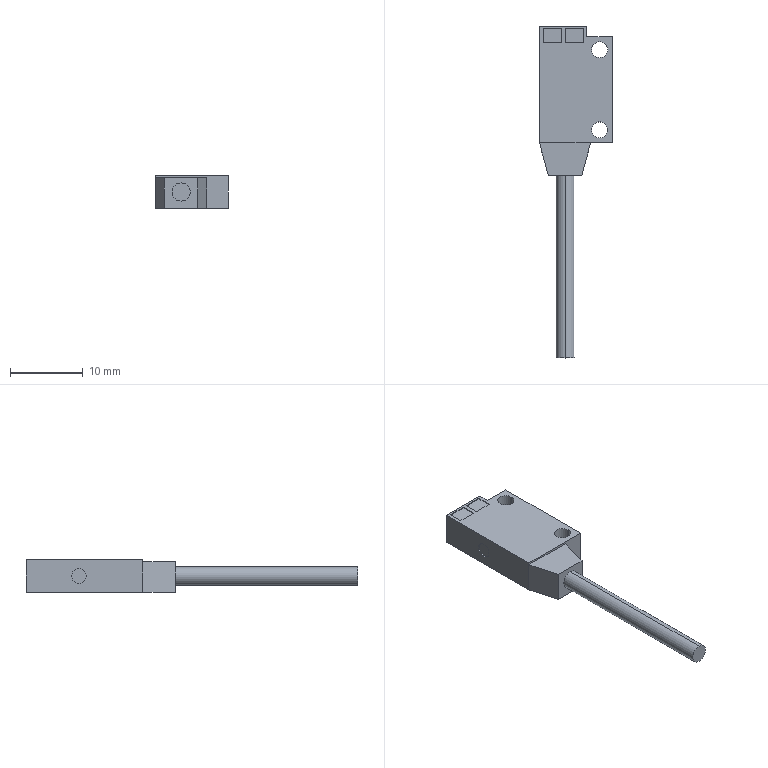Part | SolidWorks | features BaseBody 1 | 1 solid | 32 faces | box 10 x 45.5 x 4.5 mm | volume 892.741 mm3 | plane 24 | cylinder 8 | commonest cylinder face diameters 2.2 x4 2 x2 2.5 x2
STEP:
#1=CARTESIAN_POINT('',(3.5,-38.25,1.25));
#2=VERTEX_POINT('',#1);
#3=CARTESIAN_POINT('',(3.5,-38.25,-1.25));
#4=VERTEX_POINT('',#3);
#5=CARTESIAN_POINT('',(3.5,-38.25,0.));
#6=DIRECTION('',(0.,1.,0.));
#7=DIRECTION('',(0.,0.,1.));
#8=AXIS2_PLACEMENT_3D('',#5,#6,#7);
#9=CIRCLE('',#8,1.25);
#10=EDGE_CURVE('',#2,#4,#9,.T.);
#11=ORIENTED_EDGE('',*,*,#10,.F.);
#12=CARTESIAN_POINT('',(3.5,-38.25,0.));
#13=DIRECTION('',(0.,1.,0.));
#14=DIRECTION('',(0.,0.,1.));
#15=AXIS2_PLACEMENT_3D('',#12,#13,#14);
#16=CIRCLE('',#15,1.25);
#17=EDGE_CURVE('',#4,#2,#16,.T.);
#18=ORIENTED_EDGE('',*,*,#17,.F.);
#19=EDGE_LOOP('',(#11,#18));
#20=FACE_OUTER_BOUND('',#19,.T.);
#21=CARTESIAN_POINT('',(3.5,-38.25,0.));
#22=DIRECTION('',(0.,1.,0.));
#23=DIRECTION('',(1.,0.,0.));
#24=AXIS2_PLACEMENT_3D('',#21,#22,#23);
#25=PLANE('',#24);
#26=ADVANCED_FACE('',(#20),#25,.F.);
#27=ORIENTED_EDGE('',*,*,#10,.T.);
#28=CARTESIAN_POINT('',(3.5,-13.25,-1.25));
#29=VERTEX_POINT('',#28);
#30=CARTESIAN_POINT('',(3.5,-38.25,-1.25));
#31=DIRECTION('',(0.,1.,0.));
#32=VECTOR('',#31,1000.);
#33=LINE('',#30,#32);
#34=EDGE_CURVE('',#4,#29,#33,.T.);
#35=ORIENTED_EDGE('',*,*,#34,.T.);
#36=CARTESIAN_POINT('',(3.5,-13.25,1.25));
#37=VERTEX_POINT('',#36);
#38=CARTESIAN_POINT('',(3.5,-13.25,0.));
#39=DIRECTION('',(0.,1.,0.));
#40=DIRECTION('',(0.,0.,1.));
#41=AXIS2_PLACEMENT_3D('',#38,#39,#40);
#42=CIRCLE('',#41,1.25);
#43=EDGE_CURVE('',#37,#29,#42,.T.);
#44=ORIENTED_EDGE('',*,*,#43,.F.);
#45=CARTESIAN_POINT('',(3.5,-38.25,1.25));
#46=DIRECTION('',(0.,1.,0.));
#47=VECTOR('',#46,1000.);
#48=LINE('',#45,#47);
#49=EDGE_CURVE('',#2,#37,#48,.T.);
#50=ORIENTED_EDGE('',*,*,#49,.F.);
#51=EDGE_LOOP('',(#27,#35,#44,#50));
#52=FACE_OUTER_BOUND('',#51,.T.);
#53=CARTESIAN_POINT('',(3.5,-38.25,0.));
#54=DIRECTION('',(0.,1.,0.));
#55=DIRECTION('',(0.,0.,1.));
#56=AXIS2_PLACEMENT_3D('',#53,#54,#55);
#57=CYLINDRICAL_SURFACE('',#56,1.25);
#58=ADVANCED_FACE('',(#52),#57,.T.);
#59=ORIENTED_EDGE('',*,*,#34,.F.);
#60=ORIENTED_EDGE('',*,*,#17,.T.);
#61=ORIENTED_EDGE('',*,*,#49,.T.);
#62=CARTESIAN_POINT('',(3.5,-13.25,0.));
#63=DIRECTION('',(0.,1.,0.));
#64=DIRECTION('',(0.,0.,1.));
#65=AXIS2_PLACEMENT_3D('',#62,#63,#64);
#66=CIRCLE('',#65,1.25);
#67=EDGE_CURVE('',#29,#37,#66,.T.);
#68=ORIENTED_EDGE('',*,*,#67,.F.);
#69=EDGE_LOOP('',(#59,#60,#61,#68));
#70=FACE_OUTER_BOUND('',#69,.T.);
#71=CARTESIAN_POINT('',(3.5,-38.25,0.));
#72=DIRECTION('',(0.,1.,0.));
#73=DIRECTION('',(0.,0.,1.));
#74=AXIS2_PLACEMENT_3D('',#71,#72,#73);
#75=CYLINDRICAL_SURFACE('',#74,1.25);
#76=ADVANCED_FACE('',(#70),#75,.T.);
#77=CARTESIAN_POINT('',(0.1,0.,1.));
#78=VERTEX_POINT('',#77);
#79=CARTESIAN_POINT('',(0.1,0.,-1.));
#80=VERTEX_POINT('',#79);
#81=CARTESIAN_POINT('',(0.1,0.,0.));
#82=DIRECTION('',(1.,0.,0.));
#83=DIRECTION('',(0.,0.,-1.));
#84=AXIS2_PLACEMENT_3D('',#81,#82,#83);
#85=CIRCLE('',#84,1.);
#86=EDGE_CURVE('',#78,#80,#85,.T.);
#87=ORIENTED_EDGE('',*,*,#86,.F.);
#88=CARTESIAN_POINT('',(0.1,0.,0.));
#89=DIRECTION('',(1.,0.,0.));
#90=DIRECTION('',(0.,0.,-1.));
#91=AXIS2_PLACEMENT_3D('',#88,#89,#90);
#92=CIRCLE('',#91,1.);
#93=EDGE_CURVE('',#80,#78,#92,.T.);
#94=ORIENTED_EDGE('',*,*,#93,.F.);
#95=EDGE_LOOP('',(#87,#94));
#96=FACE_OUTER_BOUND('',#95,.T.);
#97=CARTESIAN_POINT('',(0.1,0.,0.));
#98=DIRECTION('',(1.,0.,0.));
#99=DIRECTION('',(0.,1.,0.));
#100=AXIS2_PLACEMENT_3D('',#97,#98,#99);
#101=PLANE('',#100);
#102=ADVANCED_FACE('',(#96),#101,.F.);
#103=ORIENTED_EDGE('',*,*,#43,.T.);
#104=ORIENTED_EDGE('',*,*,#67,.T.);
#105=EDGE_LOOP('',(#103,#104));
#106=FACE_BOUND('',#105,.T.);
#107=CARTESIAN_POINT('',(1.206,-13.25,1.95));
#108=VERTEX_POINT('',#107);
#109=CARTESIAN_POINT('',(1.206,-13.25,-2.25));
#110=VERTEX_POINT('',#109);
#111=CARTESIAN_POINT('',(1.206,-13.25,1.95));
#112=DIRECTION('',(0.,0.,-1.));
#113=VECTOR('',#112,1000.);
#114=LINE('',#111,#113);
#115=EDGE_CURVE('',#108,#110,#114,.T.);
#116=ORIENTED_EDGE('',*,*,#115,.T.);
#117=CARTESIAN_POINT('',(5.794,-13.25,-2.25));
#118=VERTEX_POINT('',#117);
#119=CARTESIAN_POINT('',(1.206,-13.25,-2.25));
#120=DIRECTION('',(1.,0.,0.));
#121=VECTOR('',#120,1000.);
#122=LINE('',#119,#121);
#123=EDGE_CURVE('',#110,#118,#122,.T.);
#124=ORIENTED_EDGE('',*,*,#123,.T.);
#125=CARTESIAN_POINT('',(5.794,-13.25,1.95));
#126=VERTEX_POINT('',#125);
#127=CARTESIAN_POINT('',(5.794,-13.25,1.95));
#128=DIRECTION('',(0.,0.,-1.));
#129=VECTOR('',#128,1000.);
#130=LINE('',#127,#129);
#131=EDGE_CURVE('',#126,#118,#130,.T.);
#132=ORIENTED_EDGE('',*,*,#131,.F.);
#133=CARTESIAN_POINT('',(1.206,-13.25,1.95));
#134=DIRECTION('',(1.,0.,0.));
#135=VECTOR('',#134,1000.);
#136=LINE('',#133,#135);
#137=EDGE_CURVE('',#108,#126,#136,.T.);
#138=ORIENTED_EDGE('',*,*,#137,.F.);
#139=EDGE_LOOP('',(#116,#124,#132,#138));
#140=FACE_OUTER_BOUND('',#139,.T.);
#141=CARTESIAN_POINT('',(1.206,-13.25,1.95));
#142=DIRECTION('',(0.,1.,0.));
#143=DIRECTION('',(1.,0.,0.));
#144=AXIS2_PLACEMENT_3D('',#141,#142,#143);
#145=PLANE('',#144);
#146=ADVANCED_FACE('',(#106,#140),#145,.F.);
#147=ORIENTED_EDGE('',*,*,#86,.T.);
#148=CARTESIAN_POINT('',(0.,0.,-1.));
#149=VERTEX_POINT('',#148);
#150=CARTESIAN_POINT('',(0.1,0.,-1.));
#151=DIRECTION('',(-1.,0.,0.));
#152=VECTOR('',#151,1000.);
#153=LINE('',#150,#152);
#154=EDGE_CURVE('',#80,#149,#153,.T.);
#155=ORIENTED_EDGE('',*,*,#154,.T.);
#156=CARTESIAN_POINT('',(0.,0.,1.));
#157=VERTEX_POINT('',#156);
#158=CARTESIAN_POINT('',(0.,0.,0.));
#159=DIRECTION('',(1.,0.,0.));
#160=DIRECTION('',(0.,0.,-1.));
#161=AXIS2_PLACEMENT_3D('',#158,#159,#160);
#162=CIRCLE('',#161,1.);
#163=EDGE_CURVE('',#157,#149,#162,.T.);
#164=ORIENTED_EDGE('',*,*,#163,.F.);
#165=CARTESIAN_POINT('',(0.1,0.,1.));
#166=DIRECTION('',(-1.,0.,0.));
#167=VECTOR('',#166,1000.);
#168=LINE('',#165,#167);
#169=EDGE_CURVE('',#78,#157,#168,.T.);
#170=ORIENTED_EDGE('',*,*,#169,.F.);
#171=EDGE_LOOP('',(#147,#155,#164,#170));
#172=FACE_OUTER_BOUND('',#171,.T.);
#173=CARTESIAN_POINT('',(0.1,0.,0.));
#174=DIRECTION('',(-1.,0.,0.));
#175=DIRECTION('',(0.,0.,1.));
#176=AXIS2_PLACEMENT_3D('',#173,#174,#175);
#177=CYLINDRICAL_SURFACE('',#176,1.);
#178=ADVANCED_FACE('',(#172),#177,.F.);
#179=CARTESIAN_POINT('',(0.,-8.75,1.95));
#180=VERTEX_POINT('',#179);
#181=CARTESIAN_POINT('',(0.,-8.75,-2.25));
#182=VERTEX_POINT('',#181);
#183=CARTESIAN_POINT('',(0.,-8.75,1.95));
#184=DIRECTION('',(0.,0.,-1.));
#185=VECTOR('',#184,1000.);
#186=LINE('',#183,#185);
#187=EDGE_CURVE('',#180,#182,#186,.T.);
#188=ORIENTED_EDGE('',*,*,#187,.T.);
#189=CARTESIAN_POINT('',(0.,-8.75,-2.25));
#190=DIRECTION('',(0.2588,-0.9659,0.));
#191=VECTOR('',#190,1000.);
#192=LINE('',#189,#191);
#193=EDGE_CURVE('',#182,#110,#192,.T.);
#194=ORIENTED_EDGE('',*,*,#193,.T.);
#195=ORIENTED_EDGE('',*,*,#115,.F.);
#196=CARTESIAN_POINT('',(0.,-8.75,1.95));
#197=DIRECTION('',(0.2588,-0.9659,0.));
#198=VECTOR('',#197,1000.);
#199=LINE('',#196,#198);
#200=EDGE_CURVE('',#180,#108,#199,.T.);
#201=ORIENTED_EDGE('',*,*,#200,.F.);
#202=EDGE_LOOP('',(#188,#194,#195,#201));
#203=FACE_OUTER_BOUND('',#202,.T.);
#204=CARTESIAN_POINT('',(0.,-8.75,1.95));
#205=DIRECTION('',(0.9659,0.2588,0.));
#206=DIRECTION('',(0.,0.,-1.));
#207=AXIS2_PLACEMENT_3D('',#204,#205,#206);
#208=PLANE('',#207);
#209=ADVANCED_FACE('',(#203),#208,.F.);
#210=ORIENTED_EDGE('',*,*,#154,.F.);
#211=ORIENTED_EDGE('',*,*,#93,.T.);
#212=ORIENTED_EDGE('',*,*,#169,.T.);
#213=CARTESIAN_POINT('',(0.,0.,0.));
#214=DIRECTION('',(1.,0.,0.));
#215=DIRECTION('',(0.,0.,-1.));
#216=AXIS2_PLACEMENT_3D('',#213,#214,#215);
#217=CIRCLE('',#216,1.);
#218=EDGE_CURVE('',#149,#157,#217,.T.);
#219=ORIENTED_EDGE('',*,*,#218,.F.);
#220=EDGE_LOOP('',(#210,#211,#212,#219));
#221=FACE_OUTER_BOUND('',#220,.T.);
#222=CARTESIAN_POINT('',(0.1,0.,0.));
#223=DIRECTION('',(-1.,0.,0.));
#224=DIRECTION('',(0.,0.,1.));
#225=AXIS2_PLACEMENT_3D('',#222,#223,#224);
#226=CYLINDRICAL_SURFACE('',#225,1.);
#227=ADVANCED_FACE('',(#221),#226,.F.);
#228=ORIENTED_EDGE('',*,*,#131,.T.);
#229=CARTESIAN_POINT('',(7.,-8.75,-2.25));
#230=VERTEX_POINT('',#229);
#231=CARTESIAN_POINT('',(5.794,-13.25,-2.25));
#232=DIRECTION('',(0.2588,0.9659,0.));
#233=VECTOR('',#232,1000.);
#234=LINE('',#231,#233);
#235=EDGE_CURVE('',#118,#230,#234,.T.);
#236=ORIENTED_EDGE('',*,*,#235,.T.);
#237=CARTESIAN_POINT('',(7.,-8.75,1.95));
#238=VERTEX_POINT('',#237);
#239=CARTESIAN_POINT('',(7.,-8.75,1.95));
#240=DIRECTION('',(0.,0.,-1.));
#241=VECTOR('',#240,1000.);
#242=LINE('',#239,#241);
#243=EDGE_CURVE('',#238,#230,#242,.T.);
#244=ORIENTED_EDGE('',*,*,#243,.F.);
#245=CARTESIAN_POINT('',(5.794,-13.25,1.95));
#246=DIRECTION('',(0.2588,0.9659,0.));
#247=VECTOR('',#246,1000.);
#248=LINE('',#245,#247);
#249=EDGE_CURVE('',#126,#238,#248,.T.);
#250=ORIENTED_EDGE('',*,*,#249,.F.);
#251=EDGE_LOOP('',(#228,#236,#244,#250));
#252=FACE_OUTER_BOUND('',#251,.T.);
#253=CARTESIAN_POINT('',(5.794,-13.25,1.95));
#254=DIRECTION('',(-0.9659,0.2588,0.));
#255=DIRECTION('',(0.,0.,1.));
#256=AXIS2_PLACEMENT_3D('',#253,#254,#255);
#257=PLANE('',#256);
#258=ADVANCED_FACE('',(#252),#257,.F.);
#259=CARTESIAN_POINT('',(7.,-8.75,1.95));
#260=DIRECTION('',(-1.,0.,0.));
#261=VECTOR('',#260,1000.);
#262=LINE('',#259,#261);
#263=EDGE_CURVE('',#238,#180,#262,.T.);
#264=ORIENTED_EDGE('',*,*,#263,.T.);
#265=ORIENTED_EDGE('',*,*,#200,.T.);
#266=ORIENTED_EDGE('',*,*,#137,.T.);
#267=ORIENTED_EDGE('',*,*,#249,.T.);
#268=EDGE_LOOP('',(#264,#265,#266,#267));
#269=FACE_OUTER_BOUND('',#268,.T.);
#270=CARTESIAN_POINT('',(0.,-8.75,1.95));
#271=DIRECTION('',(0.,0.,1.));
#272=DIRECTION('',(1.,0.,0.));
#273=AXIS2_PLACEMENT_3D('',#270,#271,#272);
#274=PLANE('',#273);
#275=ADVANCED_FACE('',(#269),#274,.T.);
#276=CARTESIAN_POINT('',(3.5,4.95,2.15));
#277=VERTEX_POINT('',#276);
#278=CARTESIAN_POINT('',(6.,4.95,2.15));
#279=VERTEX_POINT('',#278);
#280=CARTESIAN_POINT('',(6.,4.95,2.15));
#281=DIRECTION('',(1.,0.,0.));
#282=VECTOR('',#281,1000.);
#283=LINE('',#280,#282);
#284=EDGE_CURVE('',#277,#279,#283,.T.);
#285=ORIENTED_EDGE('',*,*,#284,.T.);
#286=CARTESIAN_POINT('',(6.,6.95,2.15));
#287=VERTEX_POINT('',#286);
#288=CARTESIAN_POINT('',(6.,6.95,2.15));
#289=DIRECTION('',(0.,1.,0.));
#290=VECTOR('',#289,1000.);
#291=LINE('',#288,#290);
#292=EDGE_CURVE('',#279,#287,#291,.T.);
#293=ORIENTED_EDGE('',*,*,#292,.T.);
#294=CARTESIAN_POINT('',(3.5,6.95,2.15));
#295=VERTEX_POINT('',#294);
#296=CARTESIAN_POINT('',(3.5,6.95,2.15));
#297=DIRECTION('',(-1.,0.,0.));
#298=VECTOR('',#297,1000.);
#299=LINE('',#296,#298);
#300=EDGE_CURVE('',#287,#295,#299,.T.);
#301=ORIENTED_EDGE('',*,*,#300,.T.);
#302=CARTESIAN_POINT('',(3.5,6.95,2.15));
#303=DIRECTION('',(0.,-1.,0.));
#304=VECTOR('',#303,1000.);
#305=LINE('',#302,#304);
#306=EDGE_CURVE('',#295,#277,#305,.T.);
#307=ORIENTED_EDGE('',*,*,#306,.T.);
#308=EDGE_LOOP('',(#285,#293,#301,#307));
#309=FACE_OUTER_BOUND('',#308,.T.);
#310=CARTESIAN_POINT('',(6.,4.95,2.15));
#311=DIRECTION('',(0.,0.,1.));
#312=DIRECTION('',(1.,0.,0.));
#313=AXIS2_PLACEMENT_3D('',#310,#311,#312);
#314=PLANE('',#313);
#315=ADVANCED_FACE('',(#309),#314,.T.);
#316=CARTESIAN_POINT('',(9.35,4.,-2.25));
#317=VERTEX_POINT('',#316);
#318=CARTESIAN_POINT('',(7.15,4.,-2.25));
#319=VERTEX_POINT('',#318);
#320=CARTESIAN_POINT('',(8.25,4.,-2.25));
#321=DIRECTION('',(0.,0.,-1.));
#322=DIRECTION('',(-1.,0.,0.));
#323=AXIS2_PLACEMENT_3D('',#320,#321,#322);
#324=CIRCLE('',#323,1.1);
#325=EDGE_CURVE('',#317,#319,#324,.T.);
#326=ORIENTED_EDGE('',*,*,#325,.F.);
#327=CARTESIAN_POINT('',(8.25,4.,-2.25));
#328=DIRECTION('',(0.,0.,-1.));
#329=DIRECTION('',(-1.,0.,0.));
#330=AXIS2_PLACEMENT_3D('',#327,#328,#329);
#331=CIRCLE('',#330,1.1);
#332=EDGE_CURVE('',#319,#317,#331,.T.);
#333=ORIENTED_EDGE('',*,*,#332,.F.);
#334=EDGE_LOOP('',(#326,#333));
#335=FACE_BOUND('',#334,.T.);
#336=CARTESIAN_POINT('',(9.35,-7.,-2.25));
#337=VERTEX_POINT('',#336);
#338=CARTESIAN_POINT('',(7.15,-7.,-2.25));
#339=VERTEX_POINT('',#338);
#340=CARTESIAN_POINT('',(8.25,-7.,-2.25));
#341=DIRECTION('',(0.,0.,-1.));
#342=DIRECTION('',(-1.,0.,0.));
#343=AXIS2_PLACEMENT_3D('',#340,#341,#342);
#344=CIRCLE('',#343,1.1);
#345=EDGE_CURVE('',#337,#339,#344,.T.);
#346=ORIENTED_EDGE('',*,*,#345,.F.);
#347=CARTESIAN_POINT('',(8.25,-7.,-2.25));
#348=DIRECTION('',(0.,0.,-1.));
#349=DIRECTION('',(-1.,0.,0.));
#350=AXIS2_PLACEMENT_3D('',#347,#348,#349);
#351=CIRCLE('',#350,1.1);
#352=EDGE_CURVE('',#339,#337,#351,.T.);
#353=ORIENTED_EDGE('',*,*,#352,.F.);
#354=EDGE_LOOP('',(#346,#353));
#355=FACE_BOUND('',#354,.T.);
#356=CARTESIAN_POINT('',(6.45,5.75,-2.25));
#357=VERTEX_POINT('',#356);
#358=CARTESIAN_POINT('',(6.45,7.25,-2.25));
#359=VERTEX_POINT('',#358);
#360=CARTESIAN_POINT('',(6.45,-8.75,-2.25));
#361=DIRECTION('',(0.,1.,0.));
#362=VECTOR('',#361,1000.);
#363=LINE('',#360,#362);
#364=EDGE_CURVE('',#357,#359,#363,.T.);
#365=ORIENTED_EDGE('',*,*,#364,.F.);
#366=CARTESIAN_POINT('',(10.,5.75,-2.25));
#367=VERTEX_POINT('',#366);
#368=CARTESIAN_POINT('',(10.,5.75,-2.25));
#369=DIRECTION('',(-1.,0.,0.));
#370=VECTOR('',#369,1000.);
#371=LINE('',#368,#370);
#372=EDGE_CURVE('',#367,#357,#371,.T.);
#373=ORIENTED_EDGE('',*,*,#372,.F.);
#374=CARTESIAN_POINT('',(10.,-8.75,-2.25));
#375=VERTEX_POINT('',#374);
#376=CARTESIAN_POINT('',(10.,7.25,-2.25));
#377=DIRECTION('',(0.,1.,0.));
#378=VECTOR('',#377,1000.);
#379=LINE('',#376,#378);
#380=EDGE_CURVE('',#375,#367,#379,.T.);
#381=ORIENTED_EDGE('',*,*,#380,.F.);
#382=CARTESIAN_POINT('',(10.,-8.75,-2.25));
#383=DIRECTION('',(1.,0.,0.));
#384=VECTOR('',#383,1000.);
#385=LINE('',#382,#384);
#386=EDGE_CURVE('',#230,#375,#385,.T.);
#387=ORIENTED_EDGE('',*,*,#386,.F.);
#388=ORIENTED_EDGE('',*,*,#235,.F.);
#389=ORIENTED_EDGE('',*,*,#123,.F.);
#390=ORIENTED_EDGE('',*,*,#193,.F.);
#391=CARTESIAN_POINT('',(0.,7.25,-2.25));
#392=VERTEX_POINT('',#391);
#393=CARTESIAN_POINT('',(0.,7.25,-2.25));
#394=DIRECTION('',(0.,-1.,0.));
#395=VECTOR('',#394,1000.);
#396=LINE('',#393,#395);
#397=EDGE_CURVE('',#392,#182,#396,.T.);
#398=ORIENTED_EDGE('',*,*,#397,.F.);
#399=CARTESIAN_POINT('',(10.,7.25,-2.25));
#400=DIRECTION('',(-1.,0.,0.));
#401=VECTOR('',#400,1000.);
#402=LINE('',#399,#401);
#403=EDGE_CURVE('',#359,#392,#402,.T.);
#404=ORIENTED_EDGE('',*,*,#403,.F.);
#405=EDGE_LOOP('',(#365,#373,#381,#387,#388,#389,#390,#398,#404));
#406=FACE_OUTER_BOUND('',#405,.T.);
#407=CARTESIAN_POINT('',(10.,-8.75,-2.25));
#408=DIRECTION('',(0.,0.,-1.));
#409=DIRECTION('',(0.,-1.,0.));
#410=AXIS2_PLACEMENT_3D('',#407,#408,#409);
#411=PLANE('',#410);
#412=ADVANCED_FACE('',(#335,#355,#406),#411,.T.);
#413=ORIENTED_EDGE('',*,*,#163,.T.);
#414=ORIENTED_EDGE('',*,*,#218,.T.);
#415=EDGE_LOOP('',(#413,#414));
#416=FACE_BOUND('',#415,.T.);
#417=ORIENTED_EDGE('',*,*,#397,.T.);
#418=ORIENTED_EDGE('',*,*,#187,.F.);
#419=CARTESIAN_POINT('',(0.,-8.75,2.25));
#420=VERTEX_POINT('',#419);
#421=CARTESIAN_POINT('',(0.,-8.75,2.25));
#422=DIRECTION('',(0.,0.,-1.));
#423=VECTOR('',#422,1000.);
#424=LINE('',#421,#423);
#425=EDGE_CURVE('',#420,#180,#424,.T.);
#426=ORIENTED_EDGE('',*,*,#425,.F.);
#427=CARTESIAN_POINT('',(0.,7.25,2.25));
#428=VERTEX_POINT('',#427);
#429=CARTESIAN_POINT('',(0.,7.25,2.25));
#430=DIRECTION('',(0.,-1.,0.));
#431=VECTOR('',#430,1000.);
#432=LINE('',#429,#431);
#433=EDGE_CURVE('',#428,#420,#432,.T.);
#434=ORIENTED_EDGE('',*,*,#433,.F.);
#435=CARTESIAN_POINT('',(0.,7.25,2.25));
#436=DIRECTION('',(0.,0.,-1.));
#437=VECTOR('',#436,1000.);
#438=LINE('',#435,#437);
#439=EDGE_CURVE('',#428,#392,#438,.T.);
#440=ORIENTED_EDGE('',*,*,#439,.T.);
#441=EDGE_LOOP('',(#417,#418,#426,#434,#440));
#442=FACE_OUTER_BOUND('',#441,.T.);
#443=CARTESIAN_POINT('',(0.,7.25,2.25));
#444=DIRECTION('',(1.,0.,0.));
#445=DIRECTION('',(0.,1.,0.));
#446=AXIS2_PLACEMENT_3D('',#443,#444,#445);
#447=PLANE('',#446);
#448=ADVANCED_FACE('',(#416,#442),#447,.F.);
#449=CARTESIAN_POINT('',(3.5,6.95,2.25));
#450=VERTEX_POINT('',#449);
#451=CARTESIAN_POINT('',(3.5,4.95,2.25));
#452=VERTEX_POINT('',#451);
#453=CARTESIAN_POINT('',(3.5,6.95,2.25));
#454=DIRECTION('',(0.,-1.,0.));
#455=VECTOR('',#454,1000.);
#456=LINE('',#453,#455);
#457=EDGE_CURVE('',#450,#452,#456,.T.);
#458=ORIENTED_EDGE('',*,*,#457,.T.);
#459=CARTESIAN_POINT('',(3.5,4.95,2.15));
#460=DIRECTION('',(0.,0.,1.));
#461=VECTOR('',#460,1000.);
#462=LINE('',#459,#461);
#463=EDGE_CURVE('',#277,#452,#462,.T.);
#464=ORIENTED_EDGE('',*,*,#463,.F.);
#465=ORIENTED_EDGE('',*,*,#306,.F.);
#466=CARTESIAN_POINT('',(3.5,6.95,2.15));
#467=DIRECTION('',(0.,0.,1.));
#468=VECTOR('',#467,1000.);
#469=LINE('',#466,#468);
#470=EDGE_CURVE('',#295,#450,#469,.T.);
#471=ORIENTED_EDGE('',*,*,#470,.T.);
#472=EDGE_LOOP('',(#458,#464,#465,#471));
#473=FACE_OUTER_BOUND('',#472,.T.);
#474=CARTESIAN_POINT('',(3.5,6.95,2.15));
#475=DIRECTION('',(-1.,0.,0.));
#476=DIRECTION('',(0.,1.,0.));
#477=AXIS2_PLACEMENT_3D('',#474,#475,#476);
#478=PLANE('',#477);
#479=ADVANCED_FACE('',(#473),#478,.F.);
#480=ORIENTED_EDGE('',*,*,#325,.T.);
#481=CARTESIAN_POINT('',(7.15,4.,2.25));
#482=VERTEX_POINT('',#481);
#483=CARTESIAN_POINT('',(7.15,4.,-2.25));
#484=DIRECTION('',(0.,0.,1.));
#485=VECTOR('',#484,1000.);
#486=LINE('',#483,#485);
#487=EDGE_CURVE('',#319,#482,#486,.T.);
#488=ORIENTED_EDGE('',*,*,#487,.T.);
#489=CARTESIAN_POINT('',(9.35,4.,2.25));
#490=VERTEX_POINT('',#489);
#491=CARTESIAN_POINT('',(8.25,4.,2.25));
#492=DIRECTION('',(0.,0.,-1.));
#493=DIRECTION('',(-1.,0.,0.));
#494=AXIS2_PLACEMENT_3D('',#491,#492,#493);
#495=CIRCLE('',#494,1.1);
#496=EDGE_CURVE('',#490,#482,#495,.T.);
#497=ORIENTED_EDGE('',*,*,#496,.F.);
#498=CARTESIAN_POINT('',(9.35,4.,-2.25));
#499=DIRECTION('',(0.,0.,1.));
#500=VECTOR('',#499,1000.);
#501=LINE('',#498,#500);
#502=EDGE_CURVE('',#317,#490,#501,.T.);
#503=ORIENTED_EDGE('',*,*,#502,.F.);
#504=EDGE_LOOP('',(#480,#488,#497,#503));
#505=FACE_OUTER_BOUND('',#504,.T.);
#506=CARTESIAN_POINT('',(8.25,4.,-2.25));
#507=DIRECTION('',(0.,0.,1.));
#508=DIRECTION('',(1.,0.,0.));
#509=AXIS2_PLACEMENT_3D('',#506,#507,#508);
#510=CYLINDRICAL_SURFACE('',#509,1.1);
#511=ADVANCED_FACE('',(#505),#510,.F.);
#512=CARTESIAN_POINT('',(6.,4.95,2.25));
#513=VERTEX_POINT('',#512);
#514=CARTESIAN_POINT('',(6.,4.95,2.25));
#515=DIRECTION('',(1.,0.,0.));
#516=VECTOR('',#515,1000.);
#517=LINE('',#514,#516);
#518=EDGE_CURVE('',#452,#513,#517,.T.);
#519=ORIENTED_EDGE('',*,*,#518,.T.);
#520=CARTESIAN_POINT('',(6.,4.95,2.15));
#521=DIRECTION('',(0.,0.,1.));
#522=VECTOR('',#521,1000.);
#523=LINE('',#520,#522);
#524=EDGE_CURVE('',#279,#513,#523,.T.);
#525=ORIENTED_EDGE('',*,*,#524,.F.);
#526=ORIENTED_EDGE('',*,*,#284,.F.);
#527=ORIENTED_EDGE('',*,*,#463,.T.);
#528=EDGE_LOOP('',(#519,#525,#526,#527));
#529=FACE_OUTER_BOUND('',#528,.T.);
#530=CARTESIAN_POINT('',(6.,4.95,2.15));
#531=DIRECTION('',(0.,-1.,0.));
#532=DIRECTION('',(-1.,0.,0.));
#533=AXIS2_PLACEMENT_3D('',#530,#531,#532);
#534=PLANE('',#533);
#535=ADVANCED_FACE('',(#529),#534,.F.);
#536=CARTESIAN_POINT('',(7.15,-7.,2.25));
#537=VERTEX_POINT('',#536);
#538=CARTESIAN_POINT('',(7.15,-7.,-2.25));
#539=DIRECTION('',(0.,0.,1.));
#540=VECTOR('',#539,1000.);
#541=LINE('',#538,#540);
#542=EDGE_CURVE('',#339,#537,#541,.T.);
#543=ORIENTED_EDGE('',*,*,#542,.F.);
#544=ORIENTED_EDGE('',*,*,#352,.T.);
#545=CARTESIAN_POINT('',(9.35,-7.,2.25));
#546=VERTEX_POINT('',#545);
#547=CARTESIAN_POINT('',(9.35,-7.,-2.25));
#548=DIRECTION('',(0.,0.,1.));
#549=VECTOR('',#548,1000.);
#550=LINE('',#547,#549);
#551=EDGE_CURVE('',#337,#546,#550,.T.);
#552=ORIENTED_EDGE('',*,*,#551,.T.);
#553=CARTESIAN_POINT('',(8.25,-7.,2.25));
#554=DIRECTION('',(0.,0.,-1.));
#555=DIRECTION('',(-1.,0.,0.));
#556=AXIS2_PLACEMENT_3D('',#553,#554,#555);
#557=CIRCLE('',#556,1.1);
#558=EDGE_CURVE('',#537,#546,#557,.T.);
#559=ORIENTED_EDGE('',*,*,#558,.F.);
#560=EDGE_LOOP('',(#543,#544,#552,#559));
#561=FACE_OUTER_BOUND('',#560,.T.);
#562=CARTESIAN_POINT('',(8.25,-7.,-2.25));
#563=DIRECTION('',(0.,0.,1.));
#564=DIRECTION('',(1.,0.,0.));
#565=AXIS2_PLACEMENT_3D('',#562,#563,#564);
#566=CYLINDRICAL_SURFACE('',#565,1.1);
#567=ADVANCED_FACE('',(#561),#566,.F.);
#568=ORIENTED_EDGE('',*,*,#380,.T.);
#569=CARTESIAN_POINT('',(10.,5.75,2.25));
#570=VERTEX_POINT('',#569);
#571=CARTESIAN_POINT('',(10.,5.75,-2.25));
#572=DIRECTION('',(0.,0.,1.));
#573=VECTOR('',#572,1000.);
#574=LINE('',#571,#573);
#575=EDGE_CURVE('',#367,#570,#574,.T.);
#576=ORIENTED_EDGE('',*,*,#575,.T.);
#577=CARTESIAN_POINT('',(10.,-8.75,2.25));
#578=VERTEX_POINT('',#577);
#579=CARTESIAN_POINT('',(10.,7.25,2.25));
#580=DIRECTION('',(0.,1.,0.));
#581=VECTOR('',#580,1000.);
#582=LINE('',#579,#581);
#583=EDGE_CURVE('',#578,#570,#582,.T.);
#584=ORIENTED_EDGE('',*,*,#583,.F.);
#585=CARTESIAN_POINT('',(10.,-8.75,2.25));
#586=DIRECTION('',(0.,0.,-1.));
#587=VECTOR('',#586,1000.);
#588=LINE('',#585,#587);
#589=EDGE_CURVE('',#578,#375,#588,.T.);
#590=ORIENTED_EDGE('',*,*,#589,.T.);
#591=EDGE_LOOP('',(#568,#576,#584,#590));
#592=FACE_OUTER_BOUND('',#591,.T.);
#593=CARTESIAN_POINT('',(10.,7.25,2.25));
#594=DIRECTION('',(-1.,0.,0.));
#595=DIRECTION('',(0.,1.,0.));
#596=AXIS2_PLACEMENT_3D('',#593,#594,#595);
#597=PLANE('',#596);
#598=ADVANCED_FACE('',(#592),#597,.F.);
#599=ORIENTED_EDGE('',*,*,#487,.F.);
#600=ORIENTED_EDGE('',*,*,#332,.T.);
#601=ORIENTED_EDGE('',*,*,#502,.T.);
#602=CARTESIAN_POINT('',(8.25,4.,2.25));
#603=DIRECTION('',(0.,0.,-1.));
#604=DIRECTION('',(-1.,0.,0.));
#605=AXIS2_PLACEMENT_3D('',#602,#603,#604);
#606=CIRCLE('',#605,1.1);
#607=EDGE_CURVE('',#482,#490,#606,.T.);
#608=ORIENTED_EDGE('',*,*,#607,.F.);
#609=EDGE_LOOP('',(#599,#600,#601,#608));
#610=FACE_OUTER_BOUND('',#609,.T.);
#611=CARTESIAN_POINT('',(8.25,4.,-2.25));
#612=DIRECTION('',(0.,0.,1.));
#613=DIRECTION('',(1.,0.,0.));
#614=AXIS2_PLACEMENT_3D('',#611,#612,#613);
#615=CYLINDRICAL_SURFACE('',#614,1.1);
#616=ADVANCED_FACE('',(#610),#615,.F.);
#617=ORIENTED_EDGE('',*,*,#575,.F.);
#618=ORIENTED_EDGE('',*,*,#372,.T.);
#619=CARTESIAN_POINT('',(6.45,5.75,2.25));
#620=VERTEX_POINT('',#619);
#621=CARTESIAN_POINT('',(6.45,5.75,-2.25));
#622=DIRECTION('',(0.,0.,1.));
#623=VECTOR('',#622,1000.);
#624=LINE('',#621,#623);
#625=EDGE_CURVE('',#357,#620,#624,.T.);
#626=ORIENTED_EDGE('',*,*,#625,.T.);
#627=CARTESIAN_POINT('',(10.,5.75,2.25));
#628=DIRECTION('',(-1.,0.,0.));
#629=VECTOR('',#628,1000.);
#630=LINE('',#627,#629);
#631=EDGE_CURVE('',#570,#620,#630,.T.);
#632=ORIENTED_EDGE('',*,*,#631,.F.);
#633=EDGE_LOOP('',(#617,#618,#626,#632));
#634=FACE_OUTER_BOUND('',#633,.T.);
#635=CARTESIAN_POINT('',(6.45,5.75,-2.25));
#636=DIRECTION('',(0.,-1.,0.));
#637=DIRECTION('',(0.,0.,-1.));
#638=AXIS2_PLACEMENT_3D('',#635,#636,#637);
#639=PLANE('',#638);
#640=ADVANCED_FACE('',(#634),#639,.F.);
#641=ORIENTED_EDGE('',*,*,#263,.F.);
#642=ORIENTED_EDGE('',*,*,#243,.T.);
#643=ORIENTED_EDGE('',*,*,#386,.T.);
#644=ORIENTED_EDGE('',*,*,#589,.F.);
#645=CARTESIAN_POINT('',(10.,-8.75,2.25));
#646=DIRECTION('',(1.,0.,0.));
#647=VECTOR('',#646,1000.);
#648=LINE('',#645,#647);
#649=EDGE_CURVE('',#420,#578,#648,.T.);
#650=ORIENTED_EDGE('',*,*,#649,.F.);
#651=ORIENTED_EDGE('',*,*,#425,.T.);
#652=EDGE_LOOP('',(#641,#642,#643,#644,#650,#651));
#653=FACE_OUTER_BOUND('',#652,.T.);
#654=CARTESIAN_POINT('',(10.,-8.75,2.25));
#655=DIRECTION('',(0.,1.,0.));
#656=DIRECTION('',(1.,0.,0.));
#657=AXIS2_PLACEMENT_3D('',#654,#655,#656);
#658=PLANE('',#657);
#659=ADVANCED_FACE('',(#653),#658,.F.);
#660=CARTESIAN_POINT('',(6.45,7.25,2.25));
#661=VERTEX_POINT('',#660);
#662=CARTESIAN_POINT('',(10.,7.25,2.25));
#663=DIRECTION('',(-1.,0.,0.));
#664=VECTOR('',#663,1000.);
#665=LINE('',#662,#664);
#666=EDGE_CURVE('',#661,#428,#665,.T.);
#667=ORIENTED_EDGE('',*,*,#666,.F.);
#668=CARTESIAN_POINT('',(6.45,7.25,-2.25));
#669=DIRECTION('',(0.,0.,1.));
#670=VECTOR('',#669,1000.);
#671=LINE('',#668,#670);
#672=EDGE_CURVE('',#359,#661,#671,.T.);
#673=ORIENTED_EDGE('',*,*,#672,.F.);
#674=ORIENTED_EDGE('',*,*,#403,.T.);
#675=ORIENTED_EDGE('',*,*,#439,.F.);
#676=EDGE_LOOP('',(#667,#673,#674,#675));
#677=FACE_OUTER_BOUND('',#676,.T.);
#678=CARTESIAN_POINT('',(10.,7.25,2.25));
#679=DIRECTION('',(0.,-1.,0.));
#680=DIRECTION('',(0.,0.,-1.));
#681=AXIS2_PLACEMENT_3D('',#678,#679,#680);
#682=PLANE('',#681);
#683=ADVANCED_FACE('',(#677),#682,.F.);
#684=CARTESIAN_POINT('',(6.,6.95,2.25));
#685=VERTEX_POINT('',#684);
#686=CARTESIAN_POINT('',(6.,6.95,2.25));
#687=DIRECTION('',(0.,1.,0.));
#688=VECTOR('',#687,1000.);
#689=LINE('',#686,#688);
#690=EDGE_CURVE('',#513,#685,#689,.T.);
#691=ORIENTED_EDGE('',*,*,#690,.T.);
#692=CARTESIAN_POINT('',(6.,6.95,2.15));
#693=DIRECTION('',(0.,0.,1.));
#694=VECTOR('',#693,1000.);
#695=LINE('',#692,#694);
#696=EDGE_CURVE('',#287,#685,#695,.T.);
#697=ORIENTED_EDGE('',*,*,#696,.F.);
#698=ORIENTED_EDGE('',*,*,#292,.F.);
#699=ORIENTED_EDGE('',*,*,#524,.T.);
#700=EDGE_LOOP('',(#691,#697,#698,#699));
#701=FACE_OUTER_BOUND('',#700,.T.);
#702=CARTESIAN_POINT('',(6.,6.95,2.15));
#703=DIRECTION('',(1.,0.,0.));
#704=DIRECTION('',(0.,1.,0.));
#705=AXIS2_PLACEMENT_3D('',#702,#703,#704);
#706=PLANE('',#705);
#707=ADVANCED_FACE('',(#701),#706,.F.);
#708=ORIENTED_EDGE('',*,*,#625,.F.);
#709=ORIENTED_EDGE('',*,*,#364,.T.);
#710=ORIENTED_EDGE('',*,*,#672,.T.);
#711=CARTESIAN_POINT('',(6.45,-8.75,2.25));
#712=DIRECTION('',(0.,1.,0.));
#713=VECTOR('',#712,1000.);
#714=LINE('',#711,#713);
#715=EDGE_CURVE('',#620,#661,#714,.T.);
#716=ORIENTED_EDGE('',*,*,#715,.F.);
#717=EDGE_LOOP('',(#708,#709,#710,#716));
#718=FACE_OUTER_BOUND('',#717,.T.);
#719=CARTESIAN_POINT('',(6.45,7.25,-2.25));
#720=DIRECTION('',(-1.,0.,0.));
#721=DIRECTION('',(0.,0.,1.));
#722=AXIS2_PLACEMENT_3D('',#719,#720,#721);
#723=PLANE('',#722);
#724=ADVANCED_FACE('',(#718),#723,.F.);
#725=CARTESIAN_POINT('',(3.5,6.95,2.25));
#726=DIRECTION('',(-1.,0.,0.));
#727=VECTOR('',#726,1000.);
#728=LINE('',#725,#727);
#729=EDGE_CURVE('',#685,#450,#728,.T.);
#730=ORIENTED_EDGE('',*,*,#729,.T.);
#731=ORIENTED_EDGE('',*,*,#470,.F.);
#732=ORIENTED_EDGE('',*,*,#300,.F.);
#733=ORIENTED_EDGE('',*,*,#696,.T.);
#734=EDGE_LOOP('',(#730,#731,#732,#733));
#735=FACE_OUTER_BOUND('',#734,.T.);
#736=CARTESIAN_POINT('',(3.5,6.95,2.15));
#737=DIRECTION('',(0.,1.,0.));
#738=DIRECTION('',(1.,0.,0.));
#739=AXIS2_PLACEMENT_3D('',#736,#737,#738);
#740=PLANE('',#739);
#741=ADVANCED_FACE('',(#735),#740,.F.);
#742=ORIENTED_EDGE('',*,*,#345,.T.);
#743=ORIENTED_EDGE('',*,*,#542,.T.);
#744=CARTESIAN_POINT('',(8.25,-7.,2.25));
#745=DIRECTION('',(0.,0.,-1.));
#746=DIRECTION('',(-1.,0.,0.));
#747=AXIS2_PLACEMENT_3D('',#744,#745,#746);
#748=CIRCLE('',#747,1.1);
#749=EDGE_CURVE('',#546,#537,#748,.T.);
#750=ORIENTED_EDGE('',*,*,#749,.F.);
#751=ORIENTED_EDGE('',*,*,#551,.F.);
#752=EDGE_LOOP('',(#742,#743,#750,#751));
#753=FACE_OUTER_BOUND('',#752,.T.);
#754=CARTESIAN_POINT('',(8.25,-7.,-2.25));
#755=DIRECTION('',(0.,0.,1.));
#756=DIRECTION('',(1.,0.,0.));
#757=AXIS2_PLACEMENT_3D('',#754,#755,#756);
#758=CYLINDRICAL_SURFACE('',#757,1.1);
#759=ADVANCED_FACE('',(#753),#758,.F.);
#760=ORIENTED_EDGE('',*,*,#496,.T.);
#761=ORIENTED_EDGE('',*,*,#607,.T.);
#762=EDGE_LOOP('',(#760,#761));
#763=FACE_BOUND('',#762,.T.);
#764=ORIENTED_EDGE('',*,*,#749,.T.);
#765=ORIENTED_EDGE('',*,*,#558,.T.);
#766=EDGE_LOOP('',(#764,#765));
#767=FACE_BOUND('',#766,.T.);
#768=CARTESIAN_POINT('',(0.5,6.95,2.25));
#769=VERTEX_POINT('',#768);
#770=CARTESIAN_POINT('',(0.5,4.95,2.25));
#771=VERTEX_POINT('',#770);
#772=CARTESIAN_POINT('',(0.5,6.95,2.25));
#773=DIRECTION('',(0.,-1.,0.));
#774=VECTOR('',#773,1000.);
#775=LINE('',#772,#774);
#776=EDGE_CURVE('',#769,#771,#775,.T.);
#777=ORIENTED_EDGE('',*,*,#776,.F.);
#778=CARTESIAN_POINT('',(3.,6.95,2.25));
#779=VERTEX_POINT('',#778);
#780=CARTESIAN_POINT('',(3.,6.95,2.25));
#781=DIRECTION('',(-1.,0.,0.));
#782=VECTOR('',#781,1000.);
#783=LINE('',#780,#782);
#784=EDGE_CURVE('',#779,#769,#783,.T.);
#785=ORIENTED_EDGE('',*,*,#784,.F.);
#786=CARTESIAN_POINT('',(3.,4.95,2.25));
#787=VERTEX_POINT('',#786);
#788=CARTESIAN_POINT('',(3.,4.95,2.25));
#789=DIRECTION('',(0.,1.,0.));
#790=VECTOR('',#789,1000.);
#791=LINE('',#788,#790);
#792=EDGE_CURVE('',#787,#779,#791,.T.);
#793=ORIENTED_EDGE('',*,*,#792,.F.);
#794=CARTESIAN_POINT('',(3.,4.95,2.25));
#795=DIRECTION('',(1.,0.,0.));
#796=VECTOR('',#795,1000.);
#797=LINE('',#794,#796);
#798=EDGE_CURVE('',#771,#787,#797,.T.);
#799=ORIENTED_EDGE('',*,*,#798,.F.);
#800=EDGE_LOOP('',(#777,#785,#793,#799));
#801=FACE_BOUND('',#800,.T.);
#802=ORIENTED_EDGE('',*,*,#690,.F.);
#803=ORIENTED_EDGE('',*,*,#518,.F.);
#804=ORIENTED_EDGE('',*,*,#457,.F.);
#805=ORIENTED_EDGE('',*,*,#729,.F.);
#806=EDGE_LOOP('',(#802,#803,#804,#805));
#807=FACE_BOUND('',#806,.T.);
#808=ORIENTED_EDGE('',*,*,#631,.T.);
#809=ORIENTED_EDGE('',*,*,#715,.T.);
#810=ORIENTED_EDGE('',*,*,#666,.T.);
#811=ORIENTED_EDGE('',*,*,#433,.T.);
#812=ORIENTED_EDGE('',*,*,#649,.T.);
#813=ORIENTED_EDGE('',*,*,#583,.T.);
#814=EDGE_LOOP('',(#808,#809,#810,#811,#812,#813));
#815=FACE_OUTER_BOUND('',#814,.T.);
#816=CARTESIAN_POINT('',(10.,-8.75,2.25));
#817=DIRECTION('',(0.,0.,-1.));
#818=DIRECTION('',(0.,-1.,0.));
#819=AXIS2_PLACEMENT_3D('',#816,#817,#818);
#820=PLANE('',#819);
#821=ADVANCED_FACE('',(#763,#767,#801,#807,#815),#820,.F.);
#822=ORIENTED_EDGE('',*,*,#776,.T.);
#823=CARTESIAN_POINT('',(0.5,4.95,2.15));
#824=VERTEX_POINT('',#823);
#825=CARTESIAN_POINT('',(0.5,4.95,2.15));
#826=DIRECTION('',(0.,0.,1.));
#827=VECTOR('',#826,1000.);
#828=LINE('',#825,#827);
#829=EDGE_CURVE('',#824,#771,#828,.T.);
#830=ORIENTED_EDGE('',*,*,#829,.F.);
#831=CARTESIAN_POINT('',(0.5,6.95,2.15));
#832=VERTEX_POINT('',#831);
#833=CARTESIAN_POINT('',(0.5,6.95,2.15));
#834=DIRECTION('',(0.,-1.,0.));
#835=VECTOR('',#834,1000.);
#836=LINE('',#833,#835);
#837=EDGE_CURVE('',#832,#824,#836,.T.);
#838=ORIENTED_EDGE('',*,*,#837,.F.);
#839=CARTESIAN_POINT('',(0.5,6.95,2.15));
#840=DIRECTION('',(0.,0.,1.));
#841=VECTOR('',#840,1000.);
#842=LINE('',#839,#841);
#843=EDGE_CURVE('',#832,#769,#842,.T.);
#844=ORIENTED_EDGE('',*,*,#843,.T.);
#845=EDGE_LOOP('',(#822,#830,#838,#844));
#846=FACE_OUTER_BOUND('',#845,.T.);
#847=CARTESIAN_POINT('',(0.5,6.95,2.15));
#848=DIRECTION('',(-1.,0.,0.));
#849=DIRECTION('',(0.,1.,0.));
#850=AXIS2_PLACEMENT_3D('',#847,#848,#849);
#851=PLANE('',#850);
#852=ADVANCED_FACE('',(#846),#851,.F.);
#853=ORIENTED_EDGE('',*,*,#784,.T.);
#854=ORIENTED_EDGE('',*,*,#843,.F.);
#855=CARTESIAN_POINT('',(3.,6.95,2.15));
#856=VERTEX_POINT('',#855);
#857=CARTESIAN_POINT('',(3.,6.95,2.15));
#858=DIRECTION('',(-1.,0.,0.));
#859=VECTOR('',#858,1000.);
#860=LINE('',#857,#859);
#861=EDGE_CURVE('',#856,#832,#860,.T.);
#862=ORIENTED_EDGE('',*,*,#861,.F.);
#863=CARTESIAN_POINT('',(3.,6.95,2.15));
#864=DIRECTION('',(0.,0.,1.));
#865=VECTOR('',#864,1000.);
#866=LINE('',#863,#865);
#867=EDGE_CURVE('',#856,#779,#866,.T.);
#868=ORIENTED_EDGE('',*,*,#867,.T.);
#869=EDGE_LOOP('',(#853,#854,#862,#868));
#870=FACE_OUTER_BOUND('',#869,.T.);
#871=CARTESIAN_POINT('',(3.,6.95,2.15));
#872=DIRECTION('',(0.,1.,0.));
#873=DIRECTION('',(1.,0.,0.));
#874=AXIS2_PLACEMENT_3D('',#871,#872,#873);
#875=PLANE('',#874);
#876=ADVANCED_FACE('',(#870),#875,.F.);
#877=ORIENTED_EDGE('',*,*,#798,.T.);
#878=CARTESIAN_POINT('',(3.,4.95,2.15));
#879=VERTEX_POINT('',#878);
#880=CARTESIAN_POINT('',(3.,4.95,2.15));
#881=DIRECTION('',(0.,0.,1.));
#882=VECTOR('',#881,1000.);
#883=LINE('',#880,#882);
#884=EDGE_CURVE('',#879,#787,#883,.T.);
#885=ORIENTED_EDGE('',*,*,#884,.F.);
#886=CARTESIAN_POINT('',(3.,4.95,2.15));
#887=DIRECTION('',(1.,0.,0.));
#888=VECTOR('',#887,1000.);
#889=LINE('',#886,#888);
#890=EDGE_CURVE('',#824,#879,#889,.T.);
#891=ORIENTED_EDGE('',*,*,#890,.F.);
#892=ORIENTED_EDGE('',*,*,#829,.T.);
#893=EDGE_LOOP('',(#877,#885,#891,#892));
#894=FACE_OUTER_BOUND('',#893,.T.);
#895=CARTESIAN_POINT('',(3.,4.95,2.15));
#896=DIRECTION('',(0.,-1.,0.));
#897=DIRECTION('',(0.,0.,-1.));
#898=AXIS2_PLACEMENT_3D('',#895,#896,#897);
#899=PLANE('',#898);
#900=ADVANCED_FACE('',(#894),#899,.F.);
#901=ORIENTED_EDGE('',*,*,#792,.T.);
#902=ORIENTED_EDGE('',*,*,#867,.F.);
#903=CARTESIAN_POINT('',(3.,4.95,2.15));
#904=DIRECTION('',(0.,1.,0.));
#905=VECTOR('',#904,1000.);
#906=LINE('',#903,#905);
#907=EDGE_CURVE('',#879,#856,#906,.T.);
#908=ORIENTED_EDGE('',*,*,#907,.F.);
#909=ORIENTED_EDGE('',*,*,#884,.T.);
#910=EDGE_LOOP('',(#901,#902,#908,#909));
#911=FACE_OUTER_BOUND('',#910,.T.);
#912=CARTESIAN_POINT('',(3.,4.95,2.15));
#913=DIRECTION('',(1.,0.,0.));
#914=DIRECTION('',(0.,1.,0.));
#915=AXIS2_PLACEMENT_3D('',#912,#913,#914);
#916=PLANE('',#915);
#917=ADVANCED_FACE('',(#911),#916,.F.);
#918=ORIENTED_EDGE('',*,*,#861,.T.);
#919=ORIENTED_EDGE('',*,*,#837,.T.);
#920=ORIENTED_EDGE('',*,*,#890,.T.);
#921=ORIENTED_EDGE('',*,*,#907,.T.);
#922=EDGE_LOOP('',(#918,#919,#920,#921));
#923=FACE_OUTER_BOUND('',#922,.T.);
#924=CARTESIAN_POINT('',(3.,6.95,2.15));
#925=DIRECTION('',(0.,0.,-1.));
#926=DIRECTION('',(0.,-1.,0.));
#927=AXIS2_PLACEMENT_3D('',#924,#925,#926);
#928=PLANE('',#927);
#929=ADVANCED_FACE('',(#923),#928,.F.);
#930=CLOSED_SHELL('',(#26,#58,#76,#102,#146,#178,#209,#227,#258,#275,#315,#412,#448,#479,#511,#535,#567,#598,#616,#640,#659,#683,#707,#724,#741,#759,#821,#852,#876,#900,#917,#929));
#931=MANIFOLD_SOLID_BREP('',#930);
#932=CARTESIAN_POINT('',(0.,0.,0.));
#933=DIRECTION('',(0.,0.,1.));
#934=DIRECTION('',(1.,0.,0.));
#935=AXIS2_PLACEMENT_3D('',#932,#933,#934);
#936=(LENGTH_UNIT()NAMED_UNIT(*)SI_UNIT(.MILLI.,.METRE.));
#937=UNCERTAINTY_MEASURE_WITH_UNIT(LENGTH_MEASURE(0.00001),#936,'','');
#938=(NAMED_UNIT(*)PLANE_ANGLE_UNIT()SI_UNIT($,.RADIAN.));
#939=(NAMED_UNIT(*)SI_UNIT($,.STERADIAN.)SOLID_ANGLE_UNIT());
#940=(GEOMETRIC_REPRESENTATION_CONTEXT(3)GLOBAL_UNCERTAINTY_ASSIGNED_CONTEXT((#937))GLOBAL_UNIT_ASSIGNED_CONTEXT((#936,#938,#939))REPRESENTATION_CONTEXT('',''));
#941=ADVANCED_BREP_SHAPE_REPRESENTATION('',(#931,#935),#940);